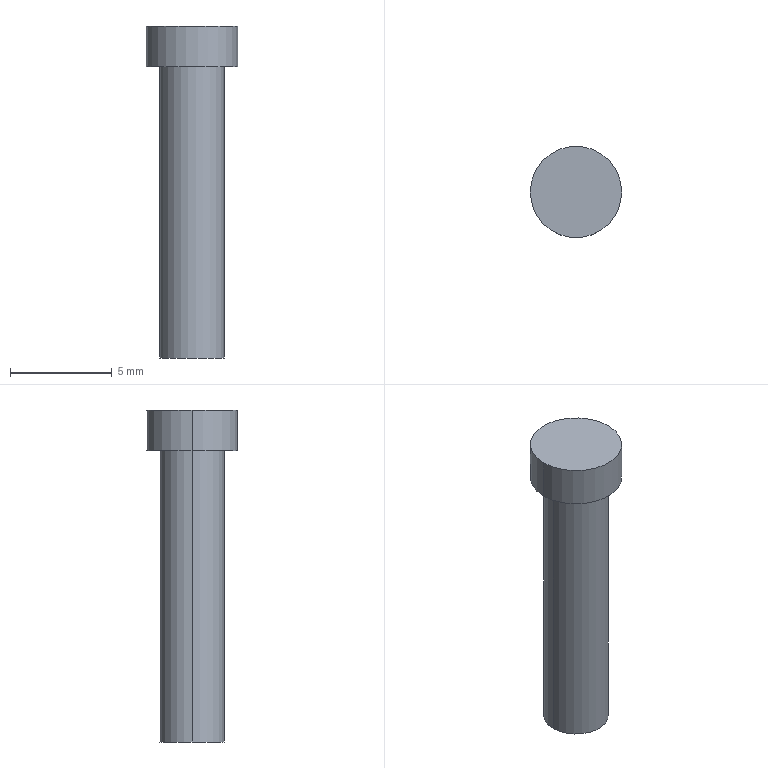Part | SolidWorks | features Extrusion 1, ICE 1 | 2 solids | 8 faces | box 4.5 x 4.5 x 16.35 mm | volume 145.78 mm3 | cylinder 4 | plane 4 | commonest cylinder face diameters 3.18 x2 4.5 x2
STEP:
#1=CARTESIAN_POINT('',(1.59,0.,14.35));
#2=VERTEX_POINT('',#1);
#3=CARTESIAN_POINT('',(-1.59,0.,14.35));
#4=VERTEX_POINT('',#3);
#5=CARTESIAN_POINT('',(0.,0.,14.35));
#6=DIRECTION('',(0.,0.,1.));
#7=DIRECTION('',(1.,0.,0.));
#8=AXIS2_PLACEMENT_3D('',#5,#6,#7);
#9=CIRCLE('',#8,1.59);
#10=EDGE_CURVE('',#2,#4,#9,.T.);
#11=ORIENTED_EDGE('',*,*,#10,.F.);
#12=CARTESIAN_POINT('',(1.59,0.,0.));
#13=VERTEX_POINT('',#12);
#14=CARTESIAN_POINT('',(1.59,0.,14.35));
#15=DIRECTION('',(0.,0.,-1.));
#16=VECTOR('',#15,1000.);
#17=LINE('',#14,#16);
#18=EDGE_CURVE('',#2,#13,#17,.T.);
#19=ORIENTED_EDGE('',*,*,#18,.T.);
#20=CARTESIAN_POINT('',(-1.59,0.,0.));
#21=VERTEX_POINT('',#20);
#22=CARTESIAN_POINT('',(0.,0.,0.));
#23=DIRECTION('',(0.,0.,1.));
#24=DIRECTION('',(1.,0.,0.));
#25=AXIS2_PLACEMENT_3D('',#22,#23,#24);
#26=CIRCLE('',#25,1.59);
#27=EDGE_CURVE('',#13,#21,#26,.T.);
#28=ORIENTED_EDGE('',*,*,#27,.T.);
#29=CARTESIAN_POINT('',(-1.59,0.,14.35));
#30=DIRECTION('',(0.,0.,-1.));
#31=VECTOR('',#30,1000.);
#32=LINE('',#29,#31);
#33=EDGE_CURVE('',#4,#21,#32,.T.);
#34=ORIENTED_EDGE('',*,*,#33,.F.);
#35=EDGE_LOOP('',(#11,#19,#28,#34));
#36=FACE_OUTER_BOUND('',#35,.T.);
#37=CARTESIAN_POINT('',(0.,0.,14.35));
#38=DIRECTION('',(0.,0.,-1.));
#39=DIRECTION('',(-1.,0.,0.));
#40=AXIS2_PLACEMENT_3D('',#37,#38,#39);
#41=CYLINDRICAL_SURFACE('',#40,1.59);
#42=ADVANCED_FACE('',(#36),#41,.T.);
#43=ORIENTED_EDGE('',*,*,#18,.F.);
#44=CARTESIAN_POINT('',(0.,0.,14.35));
#45=DIRECTION('',(0.,0.,1.));
#46=DIRECTION('',(1.,0.,0.));
#47=AXIS2_PLACEMENT_3D('',#44,#45,#46);
#48=CIRCLE('',#47,1.59);
#49=EDGE_CURVE('',#4,#2,#48,.T.);
#50=ORIENTED_EDGE('',*,*,#49,.F.);
#51=ORIENTED_EDGE('',*,*,#33,.T.);
#52=CARTESIAN_POINT('',(0.,0.,0.));
#53=DIRECTION('',(0.,0.,1.));
#54=DIRECTION('',(1.,0.,0.));
#55=AXIS2_PLACEMENT_3D('',#52,#53,#54);
#56=CIRCLE('',#55,1.59);
#57=EDGE_CURVE('',#21,#13,#56,.T.);
#58=ORIENTED_EDGE('',*,*,#57,.T.);
#59=EDGE_LOOP('',(#43,#50,#51,#58));
#60=FACE_OUTER_BOUND('',#59,.T.);
#61=CARTESIAN_POINT('',(0.,0.,14.35));
#62=DIRECTION('',(0.,0.,-1.));
#63=DIRECTION('',(-1.,0.,0.));
#64=AXIS2_PLACEMENT_3D('',#61,#62,#63);
#65=CYLINDRICAL_SURFACE('',#64,1.59);
#66=ADVANCED_FACE('',(#60),#65,.T.);
#67=ORIENTED_EDGE('',*,*,#49,.T.);
#68=ORIENTED_EDGE('',*,*,#10,.T.);
#69=EDGE_LOOP('',(#67,#68));
#70=FACE_OUTER_BOUND('',#69,.T.);
#71=CARTESIAN_POINT('',(0.,0.,14.35));
#72=DIRECTION('',(0.,0.,1.));
#73=DIRECTION('',(1.,0.,0.));
#74=AXIS2_PLACEMENT_3D('',#71,#72,#73);
#75=PLANE('',#74);
#76=ADVANCED_FACE('',(#70),#75,.T.);
#77=ORIENTED_EDGE('',*,*,#57,.F.);
#78=ORIENTED_EDGE('',*,*,#27,.F.);
#79=EDGE_LOOP('',(#77,#78));
#80=FACE_OUTER_BOUND('',#79,.T.);
#81=CARTESIAN_POINT('',(0.,0.,0.));
#82=DIRECTION('',(0.,0.,1.));
#83=DIRECTION('',(1.,0.,0.));
#84=AXIS2_PLACEMENT_3D('',#81,#82,#83);
#85=PLANE('',#84);
#86=ADVANCED_FACE('',(#80),#85,.F.);
#87=CLOSED_SHELL('',(#42,#66,#76,#86));
#88=MANIFOLD_SOLID_BREP('',#87);
#89=CARTESIAN_POINT('',(2.25,0.,16.35));
#90=VERTEX_POINT('',#89);
#91=CARTESIAN_POINT('',(-2.25,0.,16.35));
#92=VERTEX_POINT('',#91);
#93=CARTESIAN_POINT('',(0.,0.,16.35));
#94=DIRECTION('',(0.,0.,1.));
#95=DIRECTION('',(1.,0.,0.));
#96=AXIS2_PLACEMENT_3D('',#93,#94,#95);
#97=CIRCLE('',#96,2.25);
#98=EDGE_CURVE('',#90,#92,#97,.T.);
#99=ORIENTED_EDGE('',*,*,#98,.F.);
#100=CARTESIAN_POINT('',(2.25,0.,14.35));
#101=VERTEX_POINT('',#100);
#102=CARTESIAN_POINT('',(2.25,0.,16.35));
#103=DIRECTION('',(0.,0.,-1.));
#104=VECTOR('',#103,1000.);
#105=LINE('',#102,#104);
#106=EDGE_CURVE('',#90,#101,#105,.T.);
#107=ORIENTED_EDGE('',*,*,#106,.T.);
#108=CARTESIAN_POINT('',(-2.25,0.,14.35));
#109=VERTEX_POINT('',#108);
#110=CARTESIAN_POINT('',(0.,0.,14.35));
#111=DIRECTION('',(0.,0.,1.));
#112=DIRECTION('',(1.,0.,0.));
#113=AXIS2_PLACEMENT_3D('',#110,#111,#112);
#114=CIRCLE('',#113,2.25);
#115=EDGE_CURVE('',#101,#109,#114,.T.);
#116=ORIENTED_EDGE('',*,*,#115,.T.);
#117=CARTESIAN_POINT('',(-2.25,0.,16.35));
#118=DIRECTION('',(0.,0.,-1.));
#119=VECTOR('',#118,1000.);
#120=LINE('',#117,#119);
#121=EDGE_CURVE('',#92,#109,#120,.T.);
#122=ORIENTED_EDGE('',*,*,#121,.F.);
#123=EDGE_LOOP('',(#99,#107,#116,#122));
#124=FACE_OUTER_BOUND('',#123,.T.);
#125=CARTESIAN_POINT('',(0.,0.,16.35));
#126=DIRECTION('',(0.,0.,-1.));
#127=DIRECTION('',(-1.,0.,0.));
#128=AXIS2_PLACEMENT_3D('',#125,#126,#127);
#129=CYLINDRICAL_SURFACE('',#128,2.25);
#130=ADVANCED_FACE('',(#124),#129,.T.);
#131=ORIENTED_EDGE('',*,*,#106,.F.);
#132=CARTESIAN_POINT('',(0.,0.,16.35));
#133=DIRECTION('',(0.,0.,1.));
#134=DIRECTION('',(1.,0.,0.));
#135=AXIS2_PLACEMENT_3D('',#132,#133,#134);
#136=CIRCLE('',#135,2.25);
#137=EDGE_CURVE('',#92,#90,#136,.T.);
#138=ORIENTED_EDGE('',*,*,#137,.F.);
#139=ORIENTED_EDGE('',*,*,#121,.T.);
#140=CARTESIAN_POINT('',(0.,0.,14.35));
#141=DIRECTION('',(0.,0.,1.));
#142=DIRECTION('',(1.,0.,0.));
#143=AXIS2_PLACEMENT_3D('',#140,#141,#142);
#144=CIRCLE('',#143,2.25);
#145=EDGE_CURVE('',#109,#101,#144,.T.);
#146=ORIENTED_EDGE('',*,*,#145,.T.);
#147=EDGE_LOOP('',(#131,#138,#139,#146));
#148=FACE_OUTER_BOUND('',#147,.T.);
#149=CARTESIAN_POINT('',(0.,0.,16.35));
#150=DIRECTION('',(0.,0.,-1.));
#151=DIRECTION('',(-1.,0.,0.));
#152=AXIS2_PLACEMENT_3D('',#149,#150,#151);
#153=CYLINDRICAL_SURFACE('',#152,2.25);
#154=ADVANCED_FACE('',(#148),#153,.T.);
#155=ORIENTED_EDGE('',*,*,#137,.T.);
#156=ORIENTED_EDGE('',*,*,#98,.T.);
#157=EDGE_LOOP('',(#155,#156));
#158=FACE_OUTER_BOUND('',#157,.T.);
#159=CARTESIAN_POINT('',(0.,0.,16.35));
#160=DIRECTION('',(0.,0.,1.));
#161=DIRECTION('',(1.,0.,0.));
#162=AXIS2_PLACEMENT_3D('',#159,#160,#161);
#163=PLANE('',#162);
#164=ADVANCED_FACE('',(#158),#163,.T.);
#165=ORIENTED_EDGE('',*,*,#145,.F.);
#166=ORIENTED_EDGE('',*,*,#115,.F.);
#167=EDGE_LOOP('',(#165,#166));
#168=FACE_OUTER_BOUND('',#167,.T.);
#169=CARTESIAN_POINT('',(0.,0.,14.35));
#170=DIRECTION('',(0.,0.,1.));
#171=DIRECTION('',(1.,0.,0.));
#172=AXIS2_PLACEMENT_3D('',#169,#170,#171);
#173=PLANE('',#172);
#174=ADVANCED_FACE('',(#168),#173,.F.);
#175=CLOSED_SHELL('',(#130,#154,#164,#174));
#176=MANIFOLD_SOLID_BREP('',#175);
#177=CARTESIAN_POINT('',(0.,0.,0.));
#178=DIRECTION('',(0.,0.,1.));
#179=DIRECTION('',(1.,0.,0.));
#180=AXIS2_PLACEMENT_3D('',#177,#178,#179);
#181=(LENGTH_UNIT()NAMED_UNIT(*)SI_UNIT(.MILLI.,.METRE.));
#182=UNCERTAINTY_MEASURE_WITH_UNIT(LENGTH_MEASURE(0.00001),#181,'','');
#183=(NAMED_UNIT(*)PLANE_ANGLE_UNIT()SI_UNIT($,.RADIAN.));
#184=(NAMED_UNIT(*)SI_UNIT($,.STERADIAN.)SOLID_ANGLE_UNIT());
#185=(GEOMETRIC_REPRESENTATION_CONTEXT(3)GLOBAL_UNCERTAINTY_ASSIGNED_CONTEXT((#182))GLOBAL_UNIT_ASSIGNED_CONTEXT((#181,#183,#184))REPRESENTATION_CONTEXT('',''));
#186=ADVANCED_BREP_SHAPE_REPRESENTATION('',(#88,#176,#180),#185);